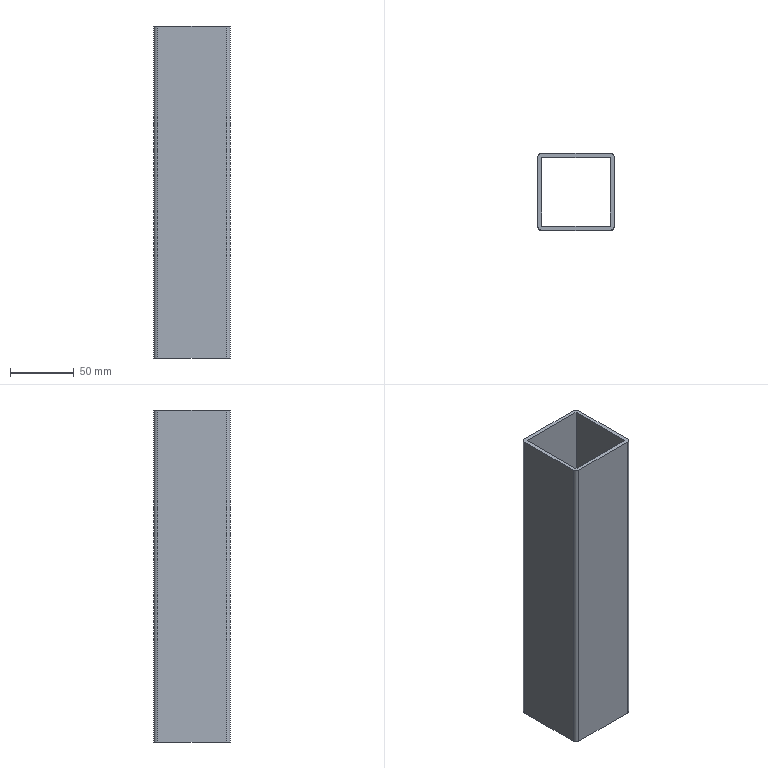Part | STEP file | X77-03110 | 1 solid | 14 faces | box 60 x 60 x 260 mm | volume 175831 mm3 | plane 10 | cylinder 4 | commonest cylinder face diameters 6 x4
STEP:
#1=CARTESIAN_POINT('',(0.,3.,260.));
#2=VERTEX_POINT('',#1);
#3=CARTESIAN_POINT('',(3.,0.,260.));
#4=VERTEX_POINT('',#3);
#5=CARTESIAN_POINT('',(3.,3.,260.));
#6=DIRECTION('',(0.,0.,1.));
#7=DIRECTION('',(1.,0.,0.));
#8=AXIS2_PLACEMENT_3D('',#5,#6,#7);
#9=CIRCLE('',#8,3.);
#10=EDGE_CURVE('',#2,#4,#9,.T.);
#11=ORIENTED_EDGE('',*,*,#10,.T.);
#12=CARTESIAN_POINT('',(57.,0.,260.));
#13=VERTEX_POINT('',#12);
#14=CARTESIAN_POINT('',(3.,0.,260.));
#15=DIRECTION('',(1.,0.,0.));
#16=VECTOR('',#15,1000.);
#17=LINE('',#14,#16);
#18=EDGE_CURVE('',#4,#13,#17,.T.);
#19=ORIENTED_EDGE('',*,*,#18,.T.);
#20=CARTESIAN_POINT('',(60.,3.,260.));
#21=VERTEX_POINT('',#20);
#22=CARTESIAN_POINT('',(57.,3.,260.));
#23=DIRECTION('',(0.,0.,1.));
#24=DIRECTION('',(1.,0.,0.));
#25=AXIS2_PLACEMENT_3D('',#22,#23,#24);
#26=CIRCLE('',#25,3.);
#27=EDGE_CURVE('',#13,#21,#26,.T.);
#28=ORIENTED_EDGE('',*,*,#27,.T.);
#29=CARTESIAN_POINT('',(60.,57.,260.));
#30=VERTEX_POINT('',#29);
#31=CARTESIAN_POINT('',(60.,3.,260.));
#32=DIRECTION('',(0.,1.,0.));
#33=VECTOR('',#32,1000.);
#34=LINE('',#31,#33);
#35=EDGE_CURVE('',#21,#30,#34,.T.);
#36=ORIENTED_EDGE('',*,*,#35,.T.);
#37=CARTESIAN_POINT('',(57.,60.,260.));
#38=VERTEX_POINT('',#37);
#39=CARTESIAN_POINT('',(57.,57.,260.));
#40=DIRECTION('',(0.,0.,1.));
#41=DIRECTION('',(1.,0.,0.));
#42=AXIS2_PLACEMENT_3D('',#39,#40,#41);
#43=CIRCLE('',#42,3.);
#44=EDGE_CURVE('',#30,#38,#43,.T.);
#45=ORIENTED_EDGE('',*,*,#44,.T.);
#46=CARTESIAN_POINT('',(3.,60.,260.));
#47=VERTEX_POINT('',#46);
#48=CARTESIAN_POINT('',(3.,60.,260.));
#49=DIRECTION('',(-1.,0.,0.));
#50=VECTOR('',#49,1000.);
#51=LINE('',#48,#50);
#52=EDGE_CURVE('',#38,#47,#51,.T.);
#53=ORIENTED_EDGE('',*,*,#52,.T.);
#54=CARTESIAN_POINT('',(0.,57.,260.));
#55=VERTEX_POINT('',#54);
#56=CARTESIAN_POINT('',(3.,57.,260.));
#57=DIRECTION('',(0.,0.,1.));
#58=DIRECTION('',(1.,0.,0.));
#59=AXIS2_PLACEMENT_3D('',#56,#57,#58);
#60=CIRCLE('',#59,3.);
#61=EDGE_CURVE('',#47,#55,#60,.T.);
#62=ORIENTED_EDGE('',*,*,#61,.T.);
#63=CARTESIAN_POINT('',(0.,3.,260.));
#64=DIRECTION('',(0.,-1.,0.));
#65=VECTOR('',#64,1000.);
#66=LINE('',#63,#65);
#67=EDGE_CURVE('',#55,#2,#66,.T.);
#68=ORIENTED_EDGE('',*,*,#67,.T.);
#69=EDGE_LOOP('',(#11,#19,#28,#36,#45,#53,#62,#68));
#70=FACE_OUTER_BOUND('',#69,.T.);
#71=CARTESIAN_POINT('',(3.,3.,260.));
#72=VERTEX_POINT('',#71);
#73=CARTESIAN_POINT('',(57.,3.,260.));
#74=VERTEX_POINT('',#73);
#75=CARTESIAN_POINT('',(3.,3.,260.));
#76=DIRECTION('',(1.,0.,0.));
#77=VECTOR('',#76,1000.);
#78=LINE('',#75,#77);
#79=EDGE_CURVE('',#72,#74,#78,.T.);
#80=ORIENTED_EDGE('',*,*,#79,.F.);
#81=CARTESIAN_POINT('',(3.,57.,260.));
#82=VERTEX_POINT('',#81);
#83=CARTESIAN_POINT('',(3.,3.,260.));
#84=DIRECTION('',(0.,-1.,0.));
#85=VECTOR('',#84,1000.);
#86=LINE('',#83,#85);
#87=EDGE_CURVE('',#82,#72,#86,.T.);
#88=ORIENTED_EDGE('',*,*,#87,.F.);
#89=CARTESIAN_POINT('',(57.,57.,260.));
#90=VERTEX_POINT('',#89);
#91=CARTESIAN_POINT('',(3.,57.,260.));
#92=DIRECTION('',(-1.,0.,0.));
#93=VECTOR('',#92,1000.);
#94=LINE('',#91,#93);
#95=EDGE_CURVE('',#90,#82,#94,.T.);
#96=ORIENTED_EDGE('',*,*,#95,.F.);
#97=CARTESIAN_POINT('',(57.,3.,260.));
#98=DIRECTION('',(0.,1.,0.));
#99=VECTOR('',#98,1000.);
#100=LINE('',#97,#99);
#101=EDGE_CURVE('',#74,#90,#100,.T.);
#102=ORIENTED_EDGE('',*,*,#101,.F.);
#103=EDGE_LOOP('',(#80,#88,#96,#102));
#104=FACE_BOUND('',#103,.T.);
#105=CARTESIAN_POINT('',(3.,3.,260.));
#106=DIRECTION('',(0.,0.,1.));
#107=DIRECTION('',(1.,0.,0.));
#108=AXIS2_PLACEMENT_3D('',#105,#106,#107);
#109=PLANE('',#108);
#110=ADVANCED_FACE('',(#70,#104),#109,.T.);
#111=CARTESIAN_POINT('',(0.,3.,0.));
#112=VERTEX_POINT('',#111);
#113=CARTESIAN_POINT('',(3.,0.,0.));
#114=VERTEX_POINT('',#113);
#115=CARTESIAN_POINT('',(3.,3.,0.));
#116=DIRECTION('',(0.,0.,1.));
#117=DIRECTION('',(1.,0.,0.));
#118=AXIS2_PLACEMENT_3D('',#115,#116,#117);
#119=CIRCLE('',#118,3.);
#120=EDGE_CURVE('',#112,#114,#119,.T.);
#121=ORIENTED_EDGE('',*,*,#120,.F.);
#122=CARTESIAN_POINT('',(0.,57.,0.));
#123=VERTEX_POINT('',#122);
#124=CARTESIAN_POINT('',(0.,3.,0.));
#125=DIRECTION('',(0.,-1.,0.));
#126=VECTOR('',#125,1000.);
#127=LINE('',#124,#126);
#128=EDGE_CURVE('',#123,#112,#127,.T.);
#129=ORIENTED_EDGE('',*,*,#128,.F.);
#130=CARTESIAN_POINT('',(3.,60.,0.));
#131=VERTEX_POINT('',#130);
#132=CARTESIAN_POINT('',(3.,57.,0.));
#133=DIRECTION('',(0.,0.,1.));
#134=DIRECTION('',(1.,0.,0.));
#135=AXIS2_PLACEMENT_3D('',#132,#133,#134);
#136=CIRCLE('',#135,3.);
#137=EDGE_CURVE('',#131,#123,#136,.T.);
#138=ORIENTED_EDGE('',*,*,#137,.F.);
#139=CARTESIAN_POINT('',(57.,60.,0.));
#140=VERTEX_POINT('',#139);
#141=CARTESIAN_POINT('',(3.,60.,0.));
#142=DIRECTION('',(-1.,0.,0.));
#143=VECTOR('',#142,1000.);
#144=LINE('',#141,#143);
#145=EDGE_CURVE('',#140,#131,#144,.T.);
#146=ORIENTED_EDGE('',*,*,#145,.F.);
#147=CARTESIAN_POINT('',(60.,57.,0.));
#148=VERTEX_POINT('',#147);
#149=CARTESIAN_POINT('',(57.,57.,0.));
#150=DIRECTION('',(0.,0.,1.));
#151=DIRECTION('',(1.,0.,0.));
#152=AXIS2_PLACEMENT_3D('',#149,#150,#151);
#153=CIRCLE('',#152,3.);
#154=EDGE_CURVE('',#148,#140,#153,.T.);
#155=ORIENTED_EDGE('',*,*,#154,.F.);
#156=CARTESIAN_POINT('',(60.,3.,0.));
#157=VERTEX_POINT('',#156);
#158=CARTESIAN_POINT('',(60.,3.,0.));
#159=DIRECTION('',(0.,1.,0.));
#160=VECTOR('',#159,1000.);
#161=LINE('',#158,#160);
#162=EDGE_CURVE('',#157,#148,#161,.T.);
#163=ORIENTED_EDGE('',*,*,#162,.F.);
#164=CARTESIAN_POINT('',(57.,0.,0.));
#165=VERTEX_POINT('',#164);
#166=CARTESIAN_POINT('',(57.,3.,0.));
#167=DIRECTION('',(0.,0.,1.));
#168=DIRECTION('',(1.,0.,0.));
#169=AXIS2_PLACEMENT_3D('',#166,#167,#168);
#170=CIRCLE('',#169,3.);
#171=EDGE_CURVE('',#165,#157,#170,.T.);
#172=ORIENTED_EDGE('',*,*,#171,.F.);
#173=CARTESIAN_POINT('',(3.,0.,0.));
#174=DIRECTION('',(1.,0.,0.));
#175=VECTOR('',#174,1000.);
#176=LINE('',#173,#175);
#177=EDGE_CURVE('',#114,#165,#176,.T.);
#178=ORIENTED_EDGE('',*,*,#177,.F.);
#179=EDGE_LOOP('',(#121,#129,#138,#146,#155,#163,#172,#178));
#180=FACE_OUTER_BOUND('',#179,.T.);
#181=CARTESIAN_POINT('',(3.,57.,0.));
#182=VERTEX_POINT('',#181);
#183=CARTESIAN_POINT('',(3.,3.,0.));
#184=VERTEX_POINT('',#183);
#185=CARTESIAN_POINT('',(3.,3.,0.));
#186=DIRECTION('',(0.,-1.,0.));
#187=VECTOR('',#186,1000.);
#188=LINE('',#185,#187);
#189=EDGE_CURVE('',#182,#184,#188,.T.);
#190=ORIENTED_EDGE('',*,*,#189,.T.);
#191=CARTESIAN_POINT('',(57.,3.,0.));
#192=VERTEX_POINT('',#191);
#193=CARTESIAN_POINT('',(3.,3.,0.));
#194=DIRECTION('',(1.,0.,0.));
#195=VECTOR('',#194,1000.);
#196=LINE('',#193,#195);
#197=EDGE_CURVE('',#184,#192,#196,.T.);
#198=ORIENTED_EDGE('',*,*,#197,.T.);
#199=CARTESIAN_POINT('',(57.,57.,0.));
#200=VERTEX_POINT('',#199);
#201=CARTESIAN_POINT('',(57.,3.,0.));
#202=DIRECTION('',(0.,1.,0.));
#203=VECTOR('',#202,1000.);
#204=LINE('',#201,#203);
#205=EDGE_CURVE('',#192,#200,#204,.T.);
#206=ORIENTED_EDGE('',*,*,#205,.T.);
#207=CARTESIAN_POINT('',(3.,57.,0.));
#208=DIRECTION('',(-1.,0.,0.));
#209=VECTOR('',#208,1000.);
#210=LINE('',#207,#209);
#211=EDGE_CURVE('',#200,#182,#210,.T.);
#212=ORIENTED_EDGE('',*,*,#211,.T.);
#213=EDGE_LOOP('',(#190,#198,#206,#212));
#214=FACE_BOUND('',#213,.T.);
#215=CARTESIAN_POINT('',(3.,3.,0.));
#216=DIRECTION('',(0.,0.,1.));
#217=DIRECTION('',(1.,0.,0.));
#218=AXIS2_PLACEMENT_3D('',#215,#216,#217);
#219=PLANE('',#218);
#220=ADVANCED_FACE('',(#180,#214),#219,.F.);
#221=ORIENTED_EDGE('',*,*,#120,.T.);
#222=CARTESIAN_POINT('',(3.,0.,260.));
#223=DIRECTION('',(0.,0.,-1.));
#224=VECTOR('',#223,1000.);
#225=LINE('',#222,#224);
#226=EDGE_CURVE('',#4,#114,#225,.T.);
#227=ORIENTED_EDGE('',*,*,#226,.F.);
#228=ORIENTED_EDGE('',*,*,#10,.F.);
#229=CARTESIAN_POINT('',(0.,3.,260.));
#230=DIRECTION('',(0.,0.,-1.));
#231=VECTOR('',#230,1000.);
#232=LINE('',#229,#231);
#233=EDGE_CURVE('',#2,#112,#232,.T.);
#234=ORIENTED_EDGE('',*,*,#233,.T.);
#235=EDGE_LOOP('',(#221,#227,#228,#234));
#236=FACE_OUTER_BOUND('',#235,.T.);
#237=CARTESIAN_POINT('',(3.,3.,260.));
#238=DIRECTION('',(0.,0.,-1.));
#239=DIRECTION('',(-1.,0.,0.));
#240=AXIS2_PLACEMENT_3D('',#237,#238,#239);
#241=CYLINDRICAL_SURFACE('',#240,3.);
#242=ADVANCED_FACE('',(#236),#241,.T.);
#243=ORIENTED_EDGE('',*,*,#177,.T.);
#244=CARTESIAN_POINT('',(57.,0.,260.));
#245=DIRECTION('',(0.,0.,-1.));
#246=VECTOR('',#245,1000.);
#247=LINE('',#244,#246);
#248=EDGE_CURVE('',#13,#165,#247,.T.);
#249=ORIENTED_EDGE('',*,*,#248,.F.);
#250=ORIENTED_EDGE('',*,*,#18,.F.);
#251=ORIENTED_EDGE('',*,*,#226,.T.);
#252=EDGE_LOOP('',(#243,#249,#250,#251));
#253=FACE_OUTER_BOUND('',#252,.T.);
#254=CARTESIAN_POINT('',(3.,0.,260.));
#255=DIRECTION('',(0.,1.,0.));
#256=DIRECTION('',(0.,0.,1.));
#257=AXIS2_PLACEMENT_3D('',#254,#255,#256);
#258=PLANE('',#257);
#259=ADVANCED_FACE('',(#253),#258,.F.);
#260=ORIENTED_EDGE('',*,*,#171,.T.);
#261=CARTESIAN_POINT('',(60.,3.,260.));
#262=DIRECTION('',(0.,0.,-1.));
#263=VECTOR('',#262,1000.);
#264=LINE('',#261,#263);
#265=EDGE_CURVE('',#21,#157,#264,.T.);
#266=ORIENTED_EDGE('',*,*,#265,.F.);
#267=ORIENTED_EDGE('',*,*,#27,.F.);
#268=ORIENTED_EDGE('',*,*,#248,.T.);
#269=EDGE_LOOP('',(#260,#266,#267,#268));
#270=FACE_OUTER_BOUND('',#269,.T.);
#271=CARTESIAN_POINT('',(57.,3.,260.));
#272=DIRECTION('',(0.,0.,-1.));
#273=DIRECTION('',(-1.,0.,0.));
#274=AXIS2_PLACEMENT_3D('',#271,#272,#273);
#275=CYLINDRICAL_SURFACE('',#274,3.);
#276=ADVANCED_FACE('',(#270),#275,.T.);
#277=ORIENTED_EDGE('',*,*,#162,.T.);
#278=CARTESIAN_POINT('',(60.,57.,260.));
#279=DIRECTION('',(0.,0.,-1.));
#280=VECTOR('',#279,1000.);
#281=LINE('',#278,#280);
#282=EDGE_CURVE('',#30,#148,#281,.T.);
#283=ORIENTED_EDGE('',*,*,#282,.F.);
#284=ORIENTED_EDGE('',*,*,#35,.F.);
#285=ORIENTED_EDGE('',*,*,#265,.T.);
#286=EDGE_LOOP('',(#277,#283,#284,#285));
#287=FACE_OUTER_BOUND('',#286,.T.);
#288=CARTESIAN_POINT('',(60.,3.,260.));
#289=DIRECTION('',(-1.,0.,0.));
#290=DIRECTION('',(0.,0.,1.));
#291=AXIS2_PLACEMENT_3D('',#288,#289,#290);
#292=PLANE('',#291);
#293=ADVANCED_FACE('',(#287),#292,.F.);
#294=ORIENTED_EDGE('',*,*,#154,.T.);
#295=CARTESIAN_POINT('',(57.,60.,260.));
#296=DIRECTION('',(0.,0.,-1.));
#297=VECTOR('',#296,1000.);
#298=LINE('',#295,#297);
#299=EDGE_CURVE('',#38,#140,#298,.T.);
#300=ORIENTED_EDGE('',*,*,#299,.F.);
#301=ORIENTED_EDGE('',*,*,#44,.F.);
#302=ORIENTED_EDGE('',*,*,#282,.T.);
#303=EDGE_LOOP('',(#294,#300,#301,#302));
#304=FACE_OUTER_BOUND('',#303,.T.);
#305=CARTESIAN_POINT('',(57.,57.,260.));
#306=DIRECTION('',(0.,0.,-1.));
#307=DIRECTION('',(-1.,0.,0.));
#308=AXIS2_PLACEMENT_3D('',#305,#306,#307);
#309=CYLINDRICAL_SURFACE('',#308,3.);
#310=ADVANCED_FACE('',(#304),#309,.T.);
#311=ORIENTED_EDGE('',*,*,#145,.T.);
#312=CARTESIAN_POINT('',(3.,60.,260.));
#313=DIRECTION('',(0.,0.,-1.));
#314=VECTOR('',#313,1000.);
#315=LINE('',#312,#314);
#316=EDGE_CURVE('',#47,#131,#315,.T.);
#317=ORIENTED_EDGE('',*,*,#316,.F.);
#318=ORIENTED_EDGE('',*,*,#52,.F.);
#319=ORIENTED_EDGE('',*,*,#299,.T.);
#320=EDGE_LOOP('',(#311,#317,#318,#319));
#321=FACE_OUTER_BOUND('',#320,.T.);
#322=CARTESIAN_POINT('',(3.,60.,260.));
#323=DIRECTION('',(0.,-1.,0.));
#324=DIRECTION('',(0.,0.,-1.));
#325=AXIS2_PLACEMENT_3D('',#322,#323,#324);
#326=PLANE('',#325);
#327=ADVANCED_FACE('',(#321),#326,.F.);
#328=ORIENTED_EDGE('',*,*,#137,.T.);
#329=CARTESIAN_POINT('',(0.,57.,260.));
#330=DIRECTION('',(0.,0.,-1.));
#331=VECTOR('',#330,1000.);
#332=LINE('',#329,#331);
#333=EDGE_CURVE('',#55,#123,#332,.T.);
#334=ORIENTED_EDGE('',*,*,#333,.F.);
#335=ORIENTED_EDGE('',*,*,#61,.F.);
#336=ORIENTED_EDGE('',*,*,#316,.T.);
#337=EDGE_LOOP('',(#328,#334,#335,#336));
#338=FACE_OUTER_BOUND('',#337,.T.);
#339=CARTESIAN_POINT('',(3.,57.,260.));
#340=DIRECTION('',(0.,0.,-1.));
#341=DIRECTION('',(-1.,0.,0.));
#342=AXIS2_PLACEMENT_3D('',#339,#340,#341);
#343=CYLINDRICAL_SURFACE('',#342,3.);
#344=ADVANCED_FACE('',(#338),#343,.T.);
#345=ORIENTED_EDGE('',*,*,#128,.T.);
#346=ORIENTED_EDGE('',*,*,#233,.F.);
#347=ORIENTED_EDGE('',*,*,#67,.F.);
#348=ORIENTED_EDGE('',*,*,#333,.T.);
#349=EDGE_LOOP('',(#345,#346,#347,#348));
#350=FACE_OUTER_BOUND('',#349,.T.);
#351=CARTESIAN_POINT('',(0.,3.,260.));
#352=DIRECTION('',(1.,0.,0.));
#353=DIRECTION('',(0.,0.,-1.));
#354=AXIS2_PLACEMENT_3D('',#351,#352,#353);
#355=PLANE('',#354);
#356=ADVANCED_FACE('',(#350),#355,.F.);
#357=ORIENTED_EDGE('',*,*,#189,.F.);
#358=CARTESIAN_POINT('',(3.,57.,260.));
#359=DIRECTION('',(0.,0.,-1.));
#360=VECTOR('',#359,1000.);
#361=LINE('',#358,#360);
#362=EDGE_CURVE('',#82,#182,#361,.T.);
#363=ORIENTED_EDGE('',*,*,#362,.F.);
#364=ORIENTED_EDGE('',*,*,#87,.T.);
#365=CARTESIAN_POINT('',(3.,3.,260.));
#366=DIRECTION('',(0.,0.,-1.));
#367=VECTOR('',#366,1000.);
#368=LINE('',#365,#367);
#369=EDGE_CURVE('',#72,#184,#368,.T.);
#370=ORIENTED_EDGE('',*,*,#369,.T.);
#371=EDGE_LOOP('',(#357,#363,#364,#370));
#372=FACE_OUTER_BOUND('',#371,.T.);
#373=CARTESIAN_POINT('',(3.,3.,260.));
#374=DIRECTION('',(1.,0.,0.));
#375=DIRECTION('',(0.,0.,-1.));
#376=AXIS2_PLACEMENT_3D('',#373,#374,#375);
#377=PLANE('',#376);
#378=ADVANCED_FACE('',(#372),#377,.T.);
#379=ORIENTED_EDGE('',*,*,#197,.F.);
#380=ORIENTED_EDGE('',*,*,#369,.F.);
#381=ORIENTED_EDGE('',*,*,#79,.T.);
#382=CARTESIAN_POINT('',(57.,3.,260.));
#383=DIRECTION('',(0.,0.,-1.));
#384=VECTOR('',#383,1000.);
#385=LINE('',#382,#384);
#386=EDGE_CURVE('',#74,#192,#385,.T.);
#387=ORIENTED_EDGE('',*,*,#386,.T.);
#388=EDGE_LOOP('',(#379,#380,#381,#387));
#389=FACE_OUTER_BOUND('',#388,.T.);
#390=CARTESIAN_POINT('',(3.,3.,260.));
#391=DIRECTION('',(0.,1.,0.));
#392=DIRECTION('',(0.,0.,1.));
#393=AXIS2_PLACEMENT_3D('',#390,#391,#392);
#394=PLANE('',#393);
#395=ADVANCED_FACE('',(#389),#394,.T.);
#396=ORIENTED_EDGE('',*,*,#205,.F.);
#397=ORIENTED_EDGE('',*,*,#386,.F.);
#398=ORIENTED_EDGE('',*,*,#101,.T.);
#399=CARTESIAN_POINT('',(57.,57.,260.));
#400=DIRECTION('',(0.,0.,-1.));
#401=VECTOR('',#400,1000.);
#402=LINE('',#399,#401);
#403=EDGE_CURVE('',#90,#200,#402,.T.);
#404=ORIENTED_EDGE('',*,*,#403,.T.);
#405=EDGE_LOOP('',(#396,#397,#398,#404));
#406=FACE_OUTER_BOUND('',#405,.T.);
#407=CARTESIAN_POINT('',(57.,3.,260.));
#408=DIRECTION('',(-1.,0.,0.));
#409=DIRECTION('',(0.,0.,1.));
#410=AXIS2_PLACEMENT_3D('',#407,#408,#409);
#411=PLANE('',#410);
#412=ADVANCED_FACE('',(#406),#411,.T.);
#413=ORIENTED_EDGE('',*,*,#211,.F.);
#414=ORIENTED_EDGE('',*,*,#403,.F.);
#415=ORIENTED_EDGE('',*,*,#95,.T.);
#416=ORIENTED_EDGE('',*,*,#362,.T.);
#417=EDGE_LOOP('',(#413,#414,#415,#416));
#418=FACE_OUTER_BOUND('',#417,.T.);
#419=CARTESIAN_POINT('',(3.,57.,260.));
#420=DIRECTION('',(0.,-1.,0.));
#421=DIRECTION('',(0.,0.,-1.));
#422=AXIS2_PLACEMENT_3D('',#419,#420,#421);
#423=PLANE('',#422);
#424=ADVANCED_FACE('',(#418),#423,.T.);
#425=CLOSED_SHELL('',(#110,#220,#242,#259,#276,#293,#310,#327,#344,#356,#378,#395,#412,#424));
#426=MANIFOLD_SOLID_BREP('',#425);
#427=CARTESIAN_POINT('',(0.,0.,0.));
#428=DIRECTION('',(0.,0.,1.));
#429=DIRECTION('',(1.,0.,0.));
#430=AXIS2_PLACEMENT_3D('',#427,#428,#429);
#431=(LENGTH_UNIT()NAMED_UNIT(*)SI_UNIT(.MILLI.,.METRE.));
#432=UNCERTAINTY_MEASURE_WITH_UNIT(LENGTH_MEASURE(0.00001),#431,'','');
#433=(NAMED_UNIT(*)PLANE_ANGLE_UNIT()SI_UNIT($,.RADIAN.));
#434=(NAMED_UNIT(*)SI_UNIT($,.STERADIAN.)SOLID_ANGLE_UNIT());
#435=(GEOMETRIC_REPRESENTATION_CONTEXT(3)GLOBAL_UNCERTAINTY_ASSIGNED_CONTEXT((#432))GLOBAL_UNIT_ASSIGNED_CONTEXT((#431,#433,#434))REPRESENTATION_CONTEXT('',''));
#436=ADVANCED_BREP_SHAPE_REPRESENTATION('',(#426,#430),#435);